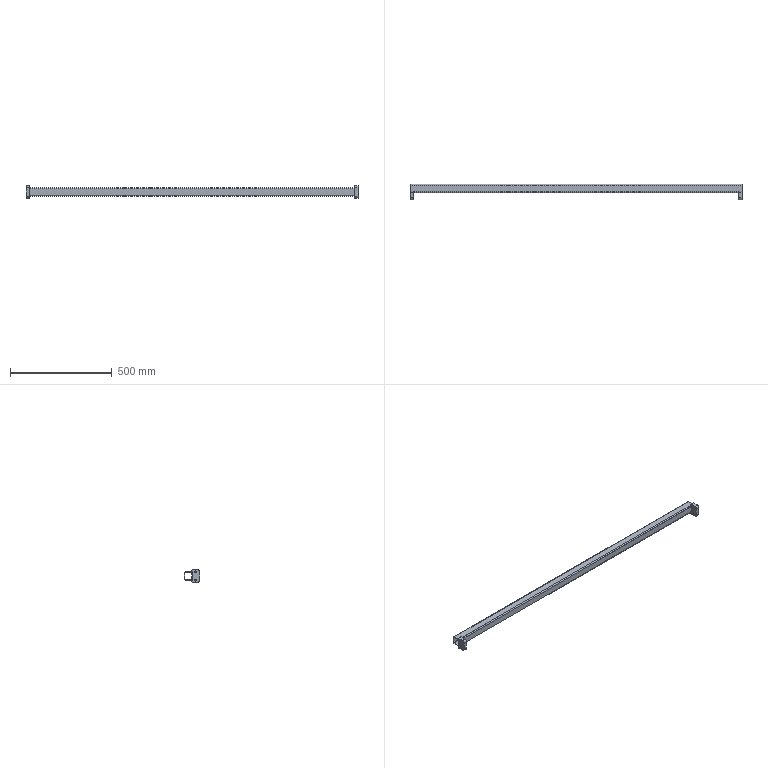Part | SolidWorks | features BaseBody 3 | 3 solids | 58 faces | box 1632 x 75 x 60 mm | volume 758697 mm3 | plane 30 | cylinder 28 | commonest cylinder face diameters 4 x8 10 x8 10.2 x8 20 x4